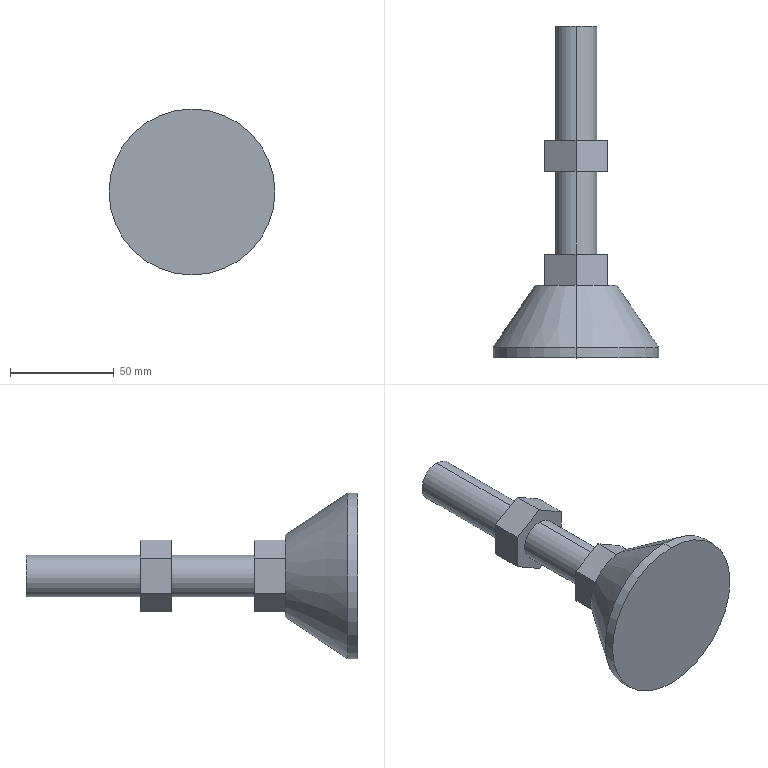Part | SolidWorks | features ICE 4, Extrusion 1 | 1 solid | 26 faces | box 80 x 160 x 80 mm | volume 165736 mm3 | plane 18 | cylinder 6 | cone 2 | commonest cylinder face diameters 20 x4 80 x2
STEP:
#1=CARTESIAN_POINT('',(0.,155.,10.));
#2=VERTEX_POINT('',#1);
#3=CARTESIAN_POINT('',(0.,155.,-10.));
#4=VERTEX_POINT('',#3);
#5=CARTESIAN_POINT('',(0.,155.,0.));
#6=DIRECTION('',(0.,1.,0.));
#7=DIRECTION('',(0.,0.,1.));
#8=AXIS2_PLACEMENT_3D('',#5,#6,#7);
#9=CIRCLE('',#8,10.);
#10=EDGE_CURVE('',#2,#4,#9,.T.);
#11=ORIENTED_EDGE('',*,*,#10,.F.);
#12=CARTESIAN_POINT('',(0.,100.,10.));
#13=VERTEX_POINT('',#12);
#14=CARTESIAN_POINT('',(0.,155.,10.));
#15=DIRECTION('',(0.,-1.,0.));
#16=VECTOR('',#15,1000.);
#17=LINE('',#14,#16);
#18=EDGE_CURVE('',#2,#13,#17,.T.);
#19=ORIENTED_EDGE('',*,*,#18,.T.);
#20=CARTESIAN_POINT('',(0.,100.,-10.));
#21=VERTEX_POINT('',#20);
#22=CARTESIAN_POINT('',(0.,100.,0.));
#23=DIRECTION('',(0.,1.,0.));
#24=DIRECTION('',(0.,0.,1.));
#25=AXIS2_PLACEMENT_3D('',#22,#23,#24);
#26=CIRCLE('',#25,10.);
#27=EDGE_CURVE('',#13,#21,#26,.T.);
#28=ORIENTED_EDGE('',*,*,#27,.T.);
#29=CARTESIAN_POINT('',(0.,155.,-10.));
#30=DIRECTION('',(0.,-1.,0.));
#31=VECTOR('',#30,1000.);
#32=LINE('',#29,#31);
#33=EDGE_CURVE('',#4,#21,#32,.T.);
#34=ORIENTED_EDGE('',*,*,#33,.F.);
#35=EDGE_LOOP('',(#11,#19,#28,#34));
#36=FACE_OUTER_BOUND('',#35,.T.);
#37=CARTESIAN_POINT('',(0.,155.,0.));
#38=DIRECTION('',(0.,-1.,0.));
#39=DIRECTION('',(0.,0.,-1.));
#40=AXIS2_PLACEMENT_3D('',#37,#38,#39);
#41=CYLINDRICAL_SURFACE('',#40,10.);
#42=ADVANCED_FACE('',(#36),#41,.T.);
#43=CARTESIAN_POINT('',(0.,-5.,-40.));
#44=VERTEX_POINT('',#43);
#45=CARTESIAN_POINT('',(0.,-5.,40.));
#46=VERTEX_POINT('',#45);
#47=CARTESIAN_POINT('',(0.,-5.,0.));
#48=DIRECTION('',(0.,-1.,0.));
#49=DIRECTION('',(0.,0.,-1.));
#50=AXIS2_PLACEMENT_3D('',#47,#48,#49);
#51=CIRCLE('',#50,40.);
#52=EDGE_CURVE('',#44,#46,#51,.T.);
#53=ORIENTED_EDGE('',*,*,#52,.F.);
#54=CARTESIAN_POINT('',(0.,0.,-40.));
#55=VERTEX_POINT('',#54);
#56=CARTESIAN_POINT('',(0.,-5.,-40.));
#57=DIRECTION('',(0.,1.,0.));
#58=VECTOR('',#57,1000.);
#59=LINE('',#56,#58);
#60=EDGE_CURVE('',#44,#55,#59,.T.);
#61=ORIENTED_EDGE('',*,*,#60,.T.);
#62=CARTESIAN_POINT('',(0.,0.,40.));
#63=VERTEX_POINT('',#62);
#64=CARTESIAN_POINT('',(0.,0.,0.));
#65=DIRECTION('',(0.,-1.,0.));
#66=DIRECTION('',(0.,0.,-1.));
#67=AXIS2_PLACEMENT_3D('',#64,#65,#66);
#68=CIRCLE('',#67,40.);
#69=EDGE_CURVE('',#55,#63,#68,.T.);
#70=ORIENTED_EDGE('',*,*,#69,.T.);
#71=CARTESIAN_POINT('',(0.,-5.,40.));
#72=DIRECTION('',(0.,1.,0.));
#73=VECTOR('',#72,1000.);
#74=LINE('',#71,#73);
#75=EDGE_CURVE('',#46,#63,#74,.T.);
#76=ORIENTED_EDGE('',*,*,#75,.F.);
#77=EDGE_LOOP('',(#53,#61,#70,#76));
#78=FACE_OUTER_BOUND('',#77,.T.);
#79=CARTESIAN_POINT('',(0.,-5.,0.));
#80=DIRECTION('',(0.,1.,0.));
#81=DIRECTION('',(0.,0.,1.));
#82=AXIS2_PLACEMENT_3D('',#79,#80,#81);
#83=CYLINDRICAL_SURFACE('',#82,40.);
#84=ADVANCED_FACE('',(#78),#83,.T.);
#85=CARTESIAN_POINT('',(0.,30.,-19.765));
#86=VERTEX_POINT('',#85);
#87=CARTESIAN_POINT('',(0.,30.,19.765));
#88=VERTEX_POINT('',#87);
#89=CARTESIAN_POINT('',(0.,30.,0.));
#90=DIRECTION('',(0.,1.,0.));
#91=DIRECTION('',(0.,0.,1.));
#92=AXIS2_PLACEMENT_3D('',#89,#90,#91);
#93=CIRCLE('',#92,19.765);
#94=EDGE_CURVE('',#86,#88,#93,.T.);
#95=ORIENTED_EDGE('',*,*,#94,.F.);
#96=CARTESIAN_POINT('',(0.,0.,-40.));
#97=DIRECTION('',(0.,-0.829,-0.5592));
#98=VECTOR('',#97,1000.);
#99=LINE('',#96,#98);
#100=EDGE_CURVE('',#86,#55,#99,.T.);
#101=ORIENTED_EDGE('',*,*,#100,.T.);
#102=CARTESIAN_POINT('',(0.,0.,0.));
#103=DIRECTION('',(0.,-1.,0.));
#104=DIRECTION('',(0.,0.,-1.));
#105=AXIS2_PLACEMENT_3D('',#102,#103,#104);
#106=CIRCLE('',#105,40.);
#107=EDGE_CURVE('',#63,#55,#106,.T.);
#108=ORIENTED_EDGE('',*,*,#107,.F.);
#109=CARTESIAN_POINT('',(0.,0.,40.));
#110=DIRECTION('',(0.,-0.829,0.5592));
#111=VECTOR('',#110,1000.);
#112=LINE('',#109,#111);
#113=EDGE_CURVE('',#88,#63,#112,.T.);
#114=ORIENTED_EDGE('',*,*,#113,.F.);
#115=EDGE_LOOP('',(#95,#101,#108,#114));
#116=FACE_OUTER_BOUND('',#115,.T.);
#117=CARTESIAN_POINT('',(0.,0.,0.));
#118=DIRECTION('',(0.,-1.,0.));
#119=DIRECTION('',(0.,0.,1.));
#120=AXIS2_PLACEMENT_3D('',#117,#118,#119);
#121=CONICAL_SURFACE('',#120,40.,0.5934);
#122=ADVANCED_FACE('',(#116),#121,.T.);
#123=CARTESIAN_POINT('',(0.,85.,10.));
#124=VERTEX_POINT('',#123);
#125=CARTESIAN_POINT('',(0.,85.,-10.));
#126=VERTEX_POINT('',#125);
#127=CARTESIAN_POINT('',(0.,85.,0.));
#128=DIRECTION('',(0.,1.,0.));
#129=DIRECTION('',(0.,0.,1.));
#130=AXIS2_PLACEMENT_3D('',#127,#128,#129);
#131=CIRCLE('',#130,10.);
#132=EDGE_CURVE('',#124,#126,#131,.T.);
#133=ORIENTED_EDGE('',*,*,#132,.F.);
#134=CARTESIAN_POINT('',(0.,45.,10.));
#135=VERTEX_POINT('',#134);
#136=CARTESIAN_POINT('',(0.,155.,10.));
#137=DIRECTION('',(0.,-1.,0.));
#138=VECTOR('',#137,1000.);
#139=LINE('',#136,#138);
#140=EDGE_CURVE('',#124,#135,#139,.T.);
#141=ORIENTED_EDGE('',*,*,#140,.T.);
#142=CARTESIAN_POINT('',(0.,45.,-10.));
#143=VERTEX_POINT('',#142);
#144=CARTESIAN_POINT('',(0.,45.,0.));
#145=DIRECTION('',(0.,1.,0.));
#146=DIRECTION('',(0.,0.,1.));
#147=AXIS2_PLACEMENT_3D('',#144,#145,#146);
#148=CIRCLE('',#147,10.);
#149=EDGE_CURVE('',#135,#143,#148,.T.);
#150=ORIENTED_EDGE('',*,*,#149,.T.);
#151=CARTESIAN_POINT('',(0.,155.,-10.));
#152=DIRECTION('',(0.,-1.,0.));
#153=VECTOR('',#152,1000.);
#154=LINE('',#151,#153);
#155=EDGE_CURVE('',#126,#143,#154,.T.);
#156=ORIENTED_EDGE('',*,*,#155,.F.);
#157=EDGE_LOOP('',(#133,#141,#150,#156));
#158=FACE_OUTER_BOUND('',#157,.T.);
#159=CARTESIAN_POINT('',(0.,155.,0.));
#160=DIRECTION('',(0.,-1.,0.));
#161=DIRECTION('',(0.,0.,-1.));
#162=AXIS2_PLACEMENT_3D('',#159,#160,#161);
#163=CYLINDRICAL_SURFACE('',#162,10.);
#164=ADVANCED_FACE('',(#158),#163,.T.);
#165=ORIENTED_EDGE('',*,*,#140,.F.);
#166=CARTESIAN_POINT('',(0.,85.,0.));
#167=DIRECTION('',(0.,1.,0.));
#168=DIRECTION('',(0.,0.,1.));
#169=AXIS2_PLACEMENT_3D('',#166,#167,#168);
#170=CIRCLE('',#169,10.);
#171=EDGE_CURVE('',#126,#124,#170,.T.);
#172=ORIENTED_EDGE('',*,*,#171,.F.);
#173=ORIENTED_EDGE('',*,*,#155,.T.);
#174=CARTESIAN_POINT('',(0.,45.,0.));
#175=DIRECTION('',(0.,1.,0.));
#176=DIRECTION('',(0.,0.,1.));
#177=AXIS2_PLACEMENT_3D('',#174,#175,#176);
#178=CIRCLE('',#177,10.);
#179=EDGE_CURVE('',#143,#135,#178,.T.);
#180=ORIENTED_EDGE('',*,*,#179,.T.);
#181=EDGE_LOOP('',(#165,#172,#173,#180));
#182=FACE_OUTER_BOUND('',#181,.T.);
#183=CARTESIAN_POINT('',(0.,155.,0.));
#184=DIRECTION('',(0.,-1.,0.));
#185=DIRECTION('',(0.,0.,-1.));
#186=AXIS2_PLACEMENT_3D('',#183,#184,#185);
#187=CYLINDRICAL_SURFACE('',#186,10.);
#188=ADVANCED_FACE('',(#182),#187,.T.);
#189=CARTESIAN_POINT('',(0.,30.,0.));
#190=DIRECTION('',(0.,1.,0.));
#191=DIRECTION('',(0.,0.,1.));
#192=AXIS2_PLACEMENT_3D('',#189,#190,#191);
#193=CIRCLE('',#192,19.765);
#194=EDGE_CURVE('',#88,#86,#193,.T.);
#195=ORIENTED_EDGE('',*,*,#194,.T.);
#196=ORIENTED_EDGE('',*,*,#94,.T.);
#197=EDGE_LOOP('',(#195,#196));
#198=FACE_OUTER_BOUND('',#197,.T.);
#199=CARTESIAN_POINT('',(15.,30.,8.66));
#200=VERTEX_POINT('',#199);
#201=CARTESIAN_POINT('',(15.,30.,-8.66));
#202=VERTEX_POINT('',#201);
#203=CARTESIAN_POINT('',(15.,30.,8.66));
#204=DIRECTION('',(0.,0.,-1.));
#205=VECTOR('',#204,1000.);
#206=LINE('',#203,#205);
#207=EDGE_CURVE('',#200,#202,#206,.T.);
#208=ORIENTED_EDGE('',*,*,#207,.F.);
#209=CARTESIAN_POINT('',(0.,30.,17.321));
#210=VERTEX_POINT('',#209);
#211=CARTESIAN_POINT('',(0.,30.,17.321));
#212=DIRECTION('',(0.866,0.,-0.5));
#213=VECTOR('',#212,1000.);
#214=LINE('',#211,#213);
#215=EDGE_CURVE('',#210,#200,#214,.T.);
#216=ORIENTED_EDGE('',*,*,#215,.F.);
#217=CARTESIAN_POINT('',(-15.,30.,8.66));
#218=VERTEX_POINT('',#217);
#219=CARTESIAN_POINT('',(-15.,30.,8.66));
#220=DIRECTION('',(0.866,0.,0.5));
#221=VECTOR('',#220,1000.);
#222=LINE('',#219,#221);
#223=EDGE_CURVE('',#218,#210,#222,.T.);
#224=ORIENTED_EDGE('',*,*,#223,.F.);
#225=CARTESIAN_POINT('',(-15.,30.,-8.66));
#226=VERTEX_POINT('',#225);
#227=CARTESIAN_POINT('',(-15.,30.,-8.66));
#228=DIRECTION('',(0.,0.,1.));
#229=VECTOR('',#228,1000.);
#230=LINE('',#227,#229);
#231=EDGE_CURVE('',#226,#218,#230,.T.);
#232=ORIENTED_EDGE('',*,*,#231,.F.);
#233=CARTESIAN_POINT('',(0.,30.,-17.321));
#234=VERTEX_POINT('',#233);
#235=CARTESIAN_POINT('',(0.,30.,-17.321));
#236=DIRECTION('',(-0.866,0.,0.5));
#237=VECTOR('',#236,1000.);
#238=LINE('',#235,#237);
#239=EDGE_CURVE('',#234,#226,#238,.T.);
#240=ORIENTED_EDGE('',*,*,#239,.F.);
#241=CARTESIAN_POINT('',(15.,30.,-8.66));
#242=DIRECTION('',(-0.866,0.,-0.5));
#243=VECTOR('',#242,1000.);
#244=LINE('',#241,#243);
#245=EDGE_CURVE('',#202,#234,#244,.T.);
#246=ORIENTED_EDGE('',*,*,#245,.F.);
#247=EDGE_LOOP('',(#208,#216,#224,#232,#240,#246));
#248=FACE_BOUND('',#247,.T.);
#249=CARTESIAN_POINT('',(0.,30.,0.));
#250=DIRECTION('',(0.,1.,0.));
#251=DIRECTION('',(0.,0.,1.));
#252=AXIS2_PLACEMENT_3D('',#249,#250,#251);
#253=PLANE('',#252);
#254=ADVANCED_FACE('',(#198,#248),#253,.T.);
#255=ORIENTED_EDGE('',*,*,#100,.F.);
#256=ORIENTED_EDGE('',*,*,#194,.F.);
#257=ORIENTED_EDGE('',*,*,#113,.T.);
#258=ORIENTED_EDGE('',*,*,#69,.F.);
#259=EDGE_LOOP('',(#255,#256,#257,#258));
#260=FACE_OUTER_BOUND('',#259,.T.);
#261=CARTESIAN_POINT('',(0.,0.,0.));
#262=DIRECTION('',(0.,-1.,0.));
#263=DIRECTION('',(0.,0.,1.));
#264=AXIS2_PLACEMENT_3D('',#261,#262,#263);
#265=CONICAL_SURFACE('',#264,40.,0.5934);
#266=ADVANCED_FACE('',(#260),#265,.T.);
#267=CARTESIAN_POINT('',(0.,45.,17.321));
#268=VERTEX_POINT('',#267);
#269=CARTESIAN_POINT('',(15.,45.,8.66));
#270=VERTEX_POINT('',#269);
#271=CARTESIAN_POINT('',(0.,45.,17.321));
#272=DIRECTION('',(0.866,0.,-0.5));
#273=VECTOR('',#272,1000.);
#274=LINE('',#271,#273);
#275=EDGE_CURVE('',#268,#270,#274,.T.);
#276=ORIENTED_EDGE('',*,*,#275,.T.);
#277=CARTESIAN_POINT('',(15.,45.,-8.66));
#278=VERTEX_POINT('',#277);
#279=CARTESIAN_POINT('',(15.,45.,8.66));
#280=DIRECTION('',(0.,0.,-1.));
#281=VECTOR('',#280,1000.);
#282=LINE('',#279,#281);
#283=EDGE_CURVE('',#270,#278,#282,.T.);
#284=ORIENTED_EDGE('',*,*,#283,.T.);
#285=CARTESIAN_POINT('',(0.,45.,-17.321));
#286=VERTEX_POINT('',#285);
#287=CARTESIAN_POINT('',(15.,45.,-8.66));
#288=DIRECTION('',(-0.866,0.,-0.5));
#289=VECTOR('',#288,1000.);
#290=LINE('',#287,#289);
#291=EDGE_CURVE('',#278,#286,#290,.T.);
#292=ORIENTED_EDGE('',*,*,#291,.T.);
#293=CARTESIAN_POINT('',(-15.,45.,-8.66));
#294=VERTEX_POINT('',#293);
#295=CARTESIAN_POINT('',(0.,45.,-17.321));
#296=DIRECTION('',(-0.866,0.,0.5));
#297=VECTOR('',#296,1000.);
#298=LINE('',#295,#297);
#299=EDGE_CURVE('',#286,#294,#298,.T.);
#300=ORIENTED_EDGE('',*,*,#299,.T.);
#301=CARTESIAN_POINT('',(-15.,45.,8.66));
#302=VERTEX_POINT('',#301);
#303=CARTESIAN_POINT('',(-15.,45.,-8.66));
#304=DIRECTION('',(0.,0.,1.));
#305=VECTOR('',#304,1000.);
#306=LINE('',#303,#305);
#307=EDGE_CURVE('',#294,#302,#306,.T.);
#308=ORIENTED_EDGE('',*,*,#307,.T.);
#309=CARTESIAN_POINT('',(-15.,45.,8.66));
#310=DIRECTION('',(0.866,0.,0.5));
#311=VECTOR('',#310,1000.);
#312=LINE('',#309,#311);
#313=EDGE_CURVE('',#302,#268,#312,.T.);
#314=ORIENTED_EDGE('',*,*,#313,.T.);
#315=EDGE_LOOP('',(#276,#284,#292,#300,#308,#314));
#316=FACE_OUTER_BOUND('',#315,.T.);
#317=ORIENTED_EDGE('',*,*,#179,.F.);
#318=ORIENTED_EDGE('',*,*,#149,.F.);
#319=EDGE_LOOP('',(#317,#318));
#320=FACE_BOUND('',#319,.T.);
#321=CARTESIAN_POINT('',(0.,45.,0.));
#322=DIRECTION('',(0.,1.,0.));
#323=DIRECTION('',(0.,0.,1.));
#324=AXIS2_PLACEMENT_3D('',#321,#322,#323);
#325=PLANE('',#324);
#326=ADVANCED_FACE('',(#316,#320),#325,.T.);
#327=ORIENTED_EDGE('',*,*,#215,.T.);
#328=CARTESIAN_POINT('',(15.,45.,8.66));
#329=DIRECTION('',(0.,-1.,0.));
#330=VECTOR('',#329,1000.);
#331=LINE('',#328,#330);
#332=EDGE_CURVE('',#270,#200,#331,.T.);
#333=ORIENTED_EDGE('',*,*,#332,.F.);
#334=ORIENTED_EDGE('',*,*,#275,.F.);
#335=CARTESIAN_POINT('',(0.,45.,17.321));
#336=DIRECTION('',(0.,-1.,0.));
#337=VECTOR('',#336,1000.);
#338=LINE('',#335,#337);
#339=EDGE_CURVE('',#268,#210,#338,.T.);
#340=ORIENTED_EDGE('',*,*,#339,.T.);
#341=EDGE_LOOP('',(#327,#333,#334,#340));
#342=FACE_OUTER_BOUND('',#341,.T.);
#343=CARTESIAN_POINT('',(0.,45.,17.321));
#344=DIRECTION('',(-0.5,0.,-0.866));
#345=DIRECTION('',(-0.866,0.,0.5));
#346=AXIS2_PLACEMENT_3D('',#343,#344,#345);
#347=PLANE('',#346);
#348=ADVANCED_FACE('',(#342),#347,.F.);
#349=ORIENTED_EDGE('',*,*,#207,.T.);
#350=CARTESIAN_POINT('',(15.,45.,-8.66));
#351=DIRECTION('',(0.,-1.,0.));
#352=VECTOR('',#351,1000.);
#353=LINE('',#350,#352);
#354=EDGE_CURVE('',#278,#202,#353,.T.);
#355=ORIENTED_EDGE('',*,*,#354,.F.);
#356=ORIENTED_EDGE('',*,*,#283,.F.);
#357=ORIENTED_EDGE('',*,*,#332,.T.);
#358=EDGE_LOOP('',(#349,#355,#356,#357));
#359=FACE_OUTER_BOUND('',#358,.T.);
#360=CARTESIAN_POINT('',(15.,45.,8.66));
#361=DIRECTION('',(-1.,0.,0.));
#362=DIRECTION('',(0.,0.,1.));
#363=AXIS2_PLACEMENT_3D('',#360,#361,#362);
#364=PLANE('',#363);
#365=ADVANCED_FACE('',(#359),#364,.F.);
#366=ORIENTED_EDGE('',*,*,#245,.T.);
#367=CARTESIAN_POINT('',(0.,45.,-17.321));
#368=DIRECTION('',(0.,-1.,0.));
#369=VECTOR('',#368,1000.);
#370=LINE('',#367,#369);
#371=EDGE_CURVE('',#286,#234,#370,.T.);
#372=ORIENTED_EDGE('',*,*,#371,.F.);
#373=ORIENTED_EDGE('',*,*,#291,.F.);
#374=ORIENTED_EDGE('',*,*,#354,.T.);
#375=EDGE_LOOP('',(#366,#372,#373,#374));
#376=FACE_OUTER_BOUND('',#375,.T.);
#377=CARTESIAN_POINT('',(15.,45.,-8.66));
#378=DIRECTION('',(-0.5,0.,0.866));
#379=DIRECTION('',(0.866,0.,0.5));
#380=AXIS2_PLACEMENT_3D('',#377,#378,#379);
#381=PLANE('',#380);
#382=ADVANCED_FACE('',(#376),#381,.F.);
#383=ORIENTED_EDGE('',*,*,#239,.T.);
#384=CARTESIAN_POINT('',(-15.,45.,-8.66));
#385=DIRECTION('',(0.,-1.,0.));
#386=VECTOR('',#385,1000.);
#387=LINE('',#384,#386);
#388=EDGE_CURVE('',#294,#226,#387,.T.);
#389=ORIENTED_EDGE('',*,*,#388,.F.);
#390=ORIENTED_EDGE('',*,*,#299,.F.);
#391=ORIENTED_EDGE('',*,*,#371,.T.);
#392=EDGE_LOOP('',(#383,#389,#390,#391));
#393=FACE_OUTER_BOUND('',#392,.T.);
#394=CARTESIAN_POINT('',(0.,45.,-17.321));
#395=DIRECTION('',(0.5,0.,0.866));
#396=DIRECTION('',(0.866,0.,-0.5));
#397=AXIS2_PLACEMENT_3D('',#394,#395,#396);
#398=PLANE('',#397);
#399=ADVANCED_FACE('',(#393),#398,.F.);
#400=ORIENTED_EDGE('',*,*,#231,.T.);
#401=CARTESIAN_POINT('',(-15.,45.,8.66));
#402=DIRECTION('',(0.,-1.,0.));
#403=VECTOR('',#402,1000.);
#404=LINE('',#401,#403);
#405=EDGE_CURVE('',#302,#218,#404,.T.);
#406=ORIENTED_EDGE('',*,*,#405,.F.);
#407=ORIENTED_EDGE('',*,*,#307,.F.);
#408=ORIENTED_EDGE('',*,*,#388,.T.);
#409=EDGE_LOOP('',(#400,#406,#407,#408));
#410=FACE_OUTER_BOUND('',#409,.T.);
#411=CARTESIAN_POINT('',(-15.,45.,-8.66));
#412=DIRECTION('',(1.,0.,0.));
#413=DIRECTION('',(0.,0.,-1.));
#414=AXIS2_PLACEMENT_3D('',#411,#412,#413);
#415=PLANE('',#414);
#416=ADVANCED_FACE('',(#410),#415,.F.);
#417=ORIENTED_EDGE('',*,*,#223,.T.);
#418=ORIENTED_EDGE('',*,*,#339,.F.);
#419=ORIENTED_EDGE('',*,*,#313,.F.);
#420=ORIENTED_EDGE('',*,*,#405,.T.);
#421=EDGE_LOOP('',(#417,#418,#419,#420));
#422=FACE_OUTER_BOUND('',#421,.T.);
#423=CARTESIAN_POINT('',(-15.,45.,8.66));
#424=DIRECTION('',(0.5,0.,-0.866));
#425=DIRECTION('',(-0.866,0.,-0.5));
#426=AXIS2_PLACEMENT_3D('',#423,#424,#425);
#427=PLANE('',#426);
#428=ADVANCED_FACE('',(#422),#427,.F.);
#429=ORIENTED_EDGE('',*,*,#60,.F.);
#430=CARTESIAN_POINT('',(0.,-5.,0.));
#431=DIRECTION('',(0.,-1.,0.));
#432=DIRECTION('',(0.,0.,-1.));
#433=AXIS2_PLACEMENT_3D('',#430,#431,#432);
#434=CIRCLE('',#433,40.);
#435=EDGE_CURVE('',#46,#44,#434,.T.);
#436=ORIENTED_EDGE('',*,*,#435,.F.);
#437=ORIENTED_EDGE('',*,*,#75,.T.);
#438=ORIENTED_EDGE('',*,*,#107,.T.);
#439=EDGE_LOOP('',(#429,#436,#437,#438));
#440=FACE_OUTER_BOUND('',#439,.T.);
#441=CARTESIAN_POINT('',(0.,-5.,0.));
#442=DIRECTION('',(0.,1.,0.));
#443=DIRECTION('',(0.,0.,1.));
#444=AXIS2_PLACEMENT_3D('',#441,#442,#443);
#445=CYLINDRICAL_SURFACE('',#444,40.);
#446=ADVANCED_FACE('',(#440),#445,.T.);
#447=ORIENTED_EDGE('',*,*,#435,.T.);
#448=ORIENTED_EDGE('',*,*,#52,.T.);
#449=EDGE_LOOP('',(#447,#448));
#450=FACE_OUTER_BOUND('',#449,.T.);
#451=CARTESIAN_POINT('',(0.,-5.,0.));
#452=DIRECTION('',(0.,-1.,0.));
#453=DIRECTION('',(0.,0.,-1.));
#454=AXIS2_PLACEMENT_3D('',#451,#452,#453);
#455=PLANE('',#454);
#456=ADVANCED_FACE('',(#450),#455,.T.);
#457=CARTESIAN_POINT('',(-15.,100.,8.66));
#458=VERTEX_POINT('',#457);
#459=CARTESIAN_POINT('',(0.,100.,17.321));
#460=VERTEX_POINT('',#459);
#461=CARTESIAN_POINT('',(-15.,100.,8.66));
#462=DIRECTION('',(0.866,0.,0.5));
#463=VECTOR('',#462,1000.);
#464=LINE('',#461,#463);
#465=EDGE_CURVE('',#458,#460,#464,.T.);
#466=ORIENTED_EDGE('',*,*,#465,.T.);
#467=CARTESIAN_POINT('',(15.,100.,8.66));
#468=VERTEX_POINT('',#467);
#469=CARTESIAN_POINT('',(0.,100.,17.321));
#470=DIRECTION('',(0.866,0.,-0.5));
#471=VECTOR('',#470,1000.);
#472=LINE('',#469,#471);
#473=EDGE_CURVE('',#460,#468,#472,.T.);
#474=ORIENTED_EDGE('',*,*,#473,.T.);
#475=CARTESIAN_POINT('',(15.,100.,-8.66));
#476=VERTEX_POINT('',#475);
#477=CARTESIAN_POINT('',(15.,100.,8.66));
#478=DIRECTION('',(0.,0.,-1.));
#479=VECTOR('',#478,1000.);
#480=LINE('',#477,#479);
#481=EDGE_CURVE('',#468,#476,#480,.T.);
#482=ORIENTED_EDGE('',*,*,#481,.T.);
#483=CARTESIAN_POINT('',(0.,100.,-17.321));
#484=VERTEX_POINT('',#483);
#485=CARTESIAN_POINT('',(15.,100.,-8.66));
#486=DIRECTION('',(-0.866,0.,-0.5));
#487=VECTOR('',#486,1000.);
#488=LINE('',#485,#487);
#489=EDGE_CURVE('',#476,#484,#488,.T.);
#490=ORIENTED_EDGE('',*,*,#489,.T.);
#491=CARTESIAN_POINT('',(-15.,100.,-8.66));
#492=VERTEX_POINT('',#491);
#493=CARTESIAN_POINT('',(0.,100.,-17.321));
#494=DIRECTION('',(-0.866,0.,0.5));
#495=VECTOR('',#494,1000.);
#496=LINE('',#493,#495);
#497=EDGE_CURVE('',#484,#492,#496,.T.);
#498=ORIENTED_EDGE('',*,*,#497,.T.);
#499=CARTESIAN_POINT('',(-15.,100.,-8.66));
#500=DIRECTION('',(0.,0.,1.));
#501=VECTOR('',#500,1000.);
#502=LINE('',#499,#501);
#503=EDGE_CURVE('',#492,#458,#502,.T.);
#504=ORIENTED_EDGE('',*,*,#503,.T.);
#505=EDGE_LOOP('',(#466,#474,#482,#490,#498,#504));
#506=FACE_OUTER_BOUND('',#505,.T.);
#507=CARTESIAN_POINT('',(0.,100.,0.));
#508=DIRECTION('',(0.,1.,0.));
#509=DIRECTION('',(0.,0.,1.));
#510=AXIS2_PLACEMENT_3D('',#507,#508,#509);
#511=CIRCLE('',#510,10.);
#512=EDGE_CURVE('',#21,#13,#511,.T.);
#513=ORIENTED_EDGE('',*,*,#512,.F.);
#514=ORIENTED_EDGE('',*,*,#27,.F.);
#515=EDGE_LOOP('',(#513,#514));
#516=FACE_BOUND('',#515,.T.);
#517=CARTESIAN_POINT('',(0.,100.,0.));
#518=DIRECTION('',(0.,1.,0.));
#519=DIRECTION('',(0.,0.,1.));
#520=AXIS2_PLACEMENT_3D('',#517,#518,#519);
#521=PLANE('',#520);
#522=ADVANCED_FACE('',(#506,#516),#521,.T.);
#523=CARTESIAN_POINT('',(-15.,85.,8.66));
#524=VERTEX_POINT('',#523);
#525=CARTESIAN_POINT('',(0.,85.,17.321));
#526=VERTEX_POINT('',#525);
#527=CARTESIAN_POINT('',(-15.,85.,8.66));
#528=DIRECTION('',(0.866,0.,0.5));
#529=VECTOR('',#528,1000.);
#530=LINE('',#527,#529);
#531=EDGE_CURVE('',#524,#526,#530,.T.);
#532=ORIENTED_EDGE('',*,*,#531,.F.);
#533=CARTESIAN_POINT('',(-15.,85.,-8.66));
#534=VERTEX_POINT('',#533);
#535=CARTESIAN_POINT('',(-15.,85.,-8.66));
#536=DIRECTION('',(0.,0.,1.));
#537=VECTOR('',#536,1000.);
#538=LINE('',#535,#537);
#539=EDGE_CURVE('',#534,#524,#538,.T.);
#540=ORIENTED_EDGE('',*,*,#539,.F.);
#541=CARTESIAN_POINT('',(0.,85.,-17.321));
#542=VERTEX_POINT('',#541);
#543=CARTESIAN_POINT('',(0.,85.,-17.321));
#544=DIRECTION('',(-0.866,0.,0.5));
#545=VECTOR('',#544,1000.);
#546=LINE('',#543,#545);
#547=EDGE_CURVE('',#542,#534,#546,.T.);
#548=ORIENTED_EDGE('',*,*,#547,.F.);
#549=CARTESIAN_POINT('',(15.,85.,-8.66));
#550=VERTEX_POINT('',#549);
#551=CARTESIAN_POINT('',(15.,85.,-8.66));
#552=DIRECTION('',(-0.866,0.,-0.5));
#553=VECTOR('',#552,1000.);
#554=LINE('',#551,#553);
#555=EDGE_CURVE('',#550,#542,#554,.T.);
#556=ORIENTED_EDGE('',*,*,#555,.F.);
#557=CARTESIAN_POINT('',(15.,85.,8.66));
#558=VERTEX_POINT('',#557);
#559=CARTESIAN_POINT('',(15.,85.,8.66));
#560=DIRECTION('',(0.,0.,-1.));
#561=VECTOR('',#560,1000.);
#562=LINE('',#559,#561);
#563=EDGE_CURVE('',#558,#550,#562,.T.);
#564=ORIENTED_EDGE('',*,*,#563,.F.);
#565=CARTESIAN_POINT('',(0.,85.,17.321));
#566=DIRECTION('',(0.866,0.,-0.5));
#567=VECTOR('',#566,1000.);
#568=LINE('',#565,#567);
#569=EDGE_CURVE('',#526,#558,#568,.T.);
#570=ORIENTED_EDGE('',*,*,#569,.F.);
#571=EDGE_LOOP('',(#532,#540,#548,#556,#564,#570));
#572=FACE_OUTER_BOUND('',#571,.T.);
#573=ORIENTED_EDGE('',*,*,#171,.T.);
#574=ORIENTED_EDGE('',*,*,#132,.T.);
#575=EDGE_LOOP('',(#573,#574));
#576=FACE_BOUND('',#575,.T.);
#577=CARTESIAN_POINT('',(0.,85.,0.));
#578=DIRECTION('',(0.,1.,0.));
#579=DIRECTION('',(0.,0.,1.));
#580=AXIS2_PLACEMENT_3D('',#577,#578,#579);
#581=PLANE('',#580);
#582=ADVANCED_FACE('',(#572,#576),#581,.F.);
#583=ORIENTED_EDGE('',*,*,#531,.T.);
#584=CARTESIAN_POINT('',(0.,100.,17.321));
#585=DIRECTION('',(0.,-1.,0.));
#586=VECTOR('',#585,1000.);
#587=LINE('',#584,#586);
#588=EDGE_CURVE('',#460,#526,#587,.T.);
#589=ORIENTED_EDGE('',*,*,#588,.F.);
#590=ORIENTED_EDGE('',*,*,#465,.F.);
#591=CARTESIAN_POINT('',(-15.,100.,8.66));
#592=DIRECTION('',(0.,-1.,0.));
#593=VECTOR('',#592,1000.);
#594=LINE('',#591,#593);
#595=EDGE_CURVE('',#458,#524,#594,.T.);
#596=ORIENTED_EDGE('',*,*,#595,.T.);
#597=EDGE_LOOP('',(#583,#589,#590,#596));
#598=FACE_OUTER_BOUND('',#597,.T.);
#599=CARTESIAN_POINT('',(-15.,100.,8.66));
#600=DIRECTION('',(0.5,0.,-0.866));
#601=DIRECTION('',(-0.866,0.,-0.5));
#602=AXIS2_PLACEMENT_3D('',#599,#600,#601);
#603=PLANE('',#602);
#604=ADVANCED_FACE('',(#598),#603,.F.);
#605=ORIENTED_EDGE('',*,*,#569,.T.);
#606=CARTESIAN_POINT('',(15.,100.,8.66));
#607=DIRECTION('',(0.,-1.,0.));
#608=VECTOR('',#607,1000.);
#609=LINE('',#606,#608);
#610=EDGE_CURVE('',#468,#558,#609,.T.);
#611=ORIENTED_EDGE('',*,*,#610,.F.);
#612=ORIENTED_EDGE('',*,*,#473,.F.);
#613=ORIENTED_EDGE('',*,*,#588,.T.);
#614=EDGE_LOOP('',(#605,#611,#612,#613));
#615=FACE_OUTER_BOUND('',#614,.T.);
#616=CARTESIAN_POINT('',(0.,100.,17.321));
#617=DIRECTION('',(-0.5,0.,-0.866));
#618=DIRECTION('',(-0.866,0.,0.5));
#619=AXIS2_PLACEMENT_3D('',#616,#617,#618);
#620=PLANE('',#619);
#621=ADVANCED_FACE('',(#615),#620,.F.);
#622=ORIENTED_EDGE('',*,*,#563,.T.);
#623=CARTESIAN_POINT('',(15.,100.,-8.66));
#624=DIRECTION('',(0.,-1.,0.));
#625=VECTOR('',#624,1000.);
#626=LINE('',#623,#625);
#627=EDGE_CURVE('',#476,#550,#626,.T.);
#628=ORIENTED_EDGE('',*,*,#627,.F.);
#629=ORIENTED_EDGE('',*,*,#481,.F.);
#630=ORIENTED_EDGE('',*,*,#610,.T.);
#631=EDGE_LOOP('',(#622,#628,#629,#630));
#632=FACE_OUTER_BOUND('',#631,.T.);
#633=CARTESIAN_POINT('',(15.,100.,8.66));
#634=DIRECTION('',(-1.,0.,0.));
#635=DIRECTION('',(0.,0.,1.));
#636=AXIS2_PLACEMENT_3D('',#633,#634,#635);
#637=PLANE('',#636);
#638=ADVANCED_FACE('',(#632),#637,.F.);
#639=ORIENTED_EDGE('',*,*,#555,.T.);
#640=CARTESIAN_POINT('',(0.,100.,-17.321));
#641=DIRECTION('',(0.,-1.,0.));
#642=VECTOR('',#641,1000.);
#643=LINE('',#640,#642);
#644=EDGE_CURVE('',#484,#542,#643,.T.);
#645=ORIENTED_EDGE('',*,*,#644,.F.);
#646=ORIENTED_EDGE('',*,*,#489,.F.);
#647=ORIENTED_EDGE('',*,*,#627,.T.);
#648=EDGE_LOOP('',(#639,#645,#646,#647));
#649=FACE_OUTER_BOUND('',#648,.T.);
#650=CARTESIAN_POINT('',(15.,100.,-8.66));
#651=DIRECTION('',(-0.5,0.,0.866));
#652=DIRECTION('',(0.866,0.,0.5));
#653=AXIS2_PLACEMENT_3D('',#650,#651,#652);
#654=PLANE('',#653);
#655=ADVANCED_FACE('',(#649),#654,.F.);
#656=ORIENTED_EDGE('',*,*,#547,.T.);
#657=CARTESIAN_POINT('',(-15.,100.,-8.66));
#658=DIRECTION('',(0.,-1.,0.));
#659=VECTOR('',#658,1000.);
#660=LINE('',#657,#659);
#661=EDGE_CURVE('',#492,#534,#660,.T.);
#662=ORIENTED_EDGE('',*,*,#661,.F.);
#663=ORIENTED_EDGE('',*,*,#497,.F.);
#664=ORIENTED_EDGE('',*,*,#644,.T.);
#665=EDGE_LOOP('',(#656,#662,#663,#664));
#666=FACE_OUTER_BOUND('',#665,.T.);
#667=CARTESIAN_POINT('',(0.,100.,-17.321));
#668=DIRECTION('',(0.5,0.,0.866));
#669=DIRECTION('',(0.866,0.,-0.5));
#670=AXIS2_PLACEMENT_3D('',#667,#668,#669);
#671=PLANE('',#670);
#672=ADVANCED_FACE('',(#666),#671,.F.);
#673=ORIENTED_EDGE('',*,*,#539,.T.);
#674=ORIENTED_EDGE('',*,*,#595,.F.);
#675=ORIENTED_EDGE('',*,*,#503,.F.);
#676=ORIENTED_EDGE('',*,*,#661,.T.);
#677=EDGE_LOOP('',(#673,#674,#675,#676));
#678=FACE_OUTER_BOUND('',#677,.T.);
#679=CARTESIAN_POINT('',(-15.,100.,-8.66));
#680=DIRECTION('',(1.,0.,0.));
#681=DIRECTION('',(0.,0.,-1.));
#682=AXIS2_PLACEMENT_3D('',#679,#680,#681);
#683=PLANE('',#682);
#684=ADVANCED_FACE('',(#678),#683,.F.);
#685=CARTESIAN_POINT('',(0.,155.,0.));
#686=DIRECTION('',(0.,1.,0.));
#687=DIRECTION('',(0.,0.,1.));
#688=AXIS2_PLACEMENT_3D('',#685,#686,#687);
#689=CIRCLE('',#688,10.);
#690=EDGE_CURVE('',#4,#2,#689,.T.);
#691=ORIENTED_EDGE('',*,*,#690,.T.);
#692=ORIENTED_EDGE('',*,*,#10,.T.);
#693=EDGE_LOOP('',(#691,#692));
#694=FACE_OUTER_BOUND('',#693,.T.);
#695=CARTESIAN_POINT('',(0.,155.,0.));
#696=DIRECTION('',(0.,1.,0.));
#697=DIRECTION('',(0.,0.,1.));
#698=AXIS2_PLACEMENT_3D('',#695,#696,#697);
#699=PLANE('',#698);
#700=ADVANCED_FACE('',(#694),#699,.T.);
#701=ORIENTED_EDGE('',*,*,#18,.F.);
#702=ORIENTED_EDGE('',*,*,#690,.F.);
#703=ORIENTED_EDGE('',*,*,#33,.T.);
#704=ORIENTED_EDGE('',*,*,#512,.T.);
#705=EDGE_LOOP('',(#701,#702,#703,#704));
#706=FACE_OUTER_BOUND('',#705,.T.);
#707=CARTESIAN_POINT('',(0.,155.,0.));
#708=DIRECTION('',(0.,-1.,0.));
#709=DIRECTION('',(0.,0.,-1.));
#710=AXIS2_PLACEMENT_3D('',#707,#708,#709);
#711=CYLINDRICAL_SURFACE('',#710,10.);
#712=ADVANCED_FACE('',(#706),#711,.T.);
#713=CLOSED_SHELL('',(#42,#84,#122,#164,#188,#254,#266,#326,#348,#365,#382,#399,#416,#428,#446,#456,#522,#582,#604,#621,#638,#655,#672,#684,#700,#712));
#714=MANIFOLD_SOLID_BREP('',#713);
#715=CARTESIAN_POINT('',(0.,0.,0.));
#716=DIRECTION('',(0.,0.,1.));
#717=DIRECTION('',(1.,0.,0.));
#718=AXIS2_PLACEMENT_3D('',#715,#716,#717);
#719=(LENGTH_UNIT()NAMED_UNIT(*)SI_UNIT(.MILLI.,.METRE.));
#720=UNCERTAINTY_MEASURE_WITH_UNIT(LENGTH_MEASURE(0.00001),#719,'','');
#721=(NAMED_UNIT(*)PLANE_ANGLE_UNIT()SI_UNIT($,.RADIAN.));
#722=(NAMED_UNIT(*)SI_UNIT($,.STERADIAN.)SOLID_ANGLE_UNIT());
#723=(GEOMETRIC_REPRESENTATION_CONTEXT(3)GLOBAL_UNCERTAINTY_ASSIGNED_CONTEXT((#720))GLOBAL_UNIT_ASSIGNED_CONTEXT((#719,#721,#722))REPRESENTATION_CONTEXT('',''));
#724=ADVANCED_BREP_SHAPE_REPRESENTATION('',(#714,#718),#723);